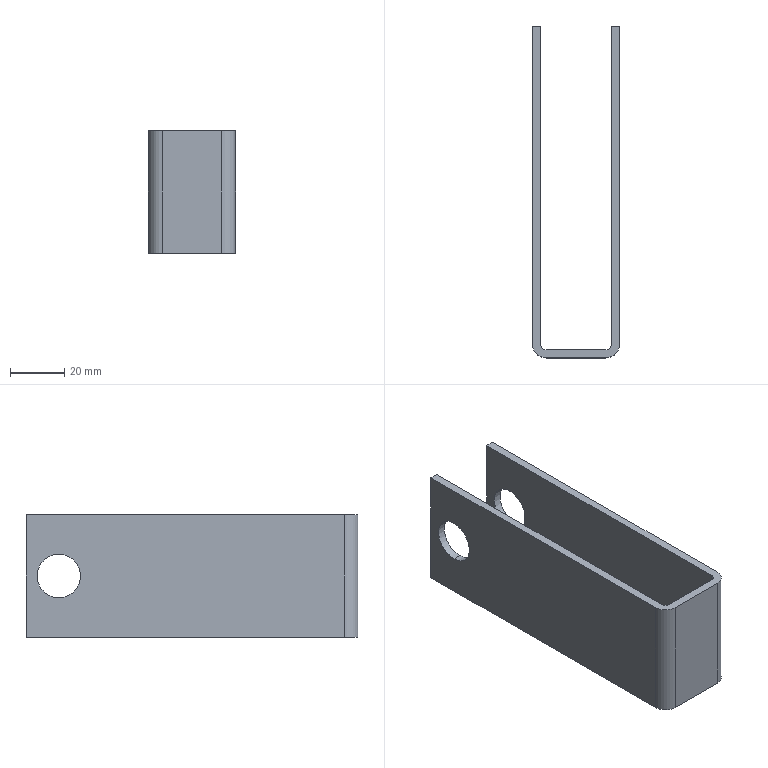Part | SolidWorks | features Extrusion 1, ICE 1 | 1 solid | 18 faces | box 32 x 122 x 45 mm | volume 34838 mm3 | plane 10 | cylinder 8 | commonest cylinder face diameters 16 x4 4 x2 10 x2
STEP:
#1=CARTESIAN_POINT('',(29.,-12.,30.5));
#2=VERTEX_POINT('',#1);
#3=CARTESIAN_POINT('',(29.,-12.,14.5));
#4=VERTEX_POINT('',#3);
#5=CARTESIAN_POINT('',(29.,-12.,22.5));
#6=DIRECTION('',(1.,0.,0.));
#7=DIRECTION('',(0.,1.,0.));
#8=AXIS2_PLACEMENT_3D('',#5,#6,#7);
#9=CIRCLE('',#8,8.);
#10=EDGE_CURVE('',#2,#4,#9,.T.);
#11=ORIENTED_EDGE('',*,*,#10,.F.);
#12=CARTESIAN_POINT('',(32.,-12.,30.5));
#13=VERTEX_POINT('',#12);
#14=CARTESIAN_POINT('',(0.,-12.,30.5));
#15=DIRECTION('',(1.,0.,0.));
#16=VECTOR('',#15,1000.);
#17=LINE('',#14,#16);
#18=EDGE_CURVE('',#2,#13,#17,.T.);
#19=ORIENTED_EDGE('',*,*,#18,.T.);
#20=CARTESIAN_POINT('',(32.,-12.,14.5));
#21=VERTEX_POINT('',#20);
#22=CARTESIAN_POINT('',(32.,-12.,22.5));
#23=DIRECTION('',(1.,0.,0.));
#24=DIRECTION('',(0.,0.,-1.));
#25=AXIS2_PLACEMENT_3D('',#22,#23,#24);
#26=CIRCLE('',#25,8.);
#27=EDGE_CURVE('',#13,#21,#26,.T.);
#28=ORIENTED_EDGE('',*,*,#27,.T.);
#29=CARTESIAN_POINT('',(0.,-12.,14.5));
#30=DIRECTION('',(1.,0.,0.));
#31=VECTOR('',#30,1000.);
#32=LINE('',#29,#31);
#33=EDGE_CURVE('',#4,#21,#32,.T.);
#34=ORIENTED_EDGE('',*,*,#33,.F.);
#35=EDGE_LOOP('',(#11,#19,#28,#34));
#36=FACE_OUTER_BOUND('',#35,.T.);
#37=CARTESIAN_POINT('',(0.,-12.,22.5));
#38=DIRECTION('',(1.,0.,0.));
#39=DIRECTION('',(0.,0.,-1.));
#40=AXIS2_PLACEMENT_3D('',#37,#38,#39);
#41=CYLINDRICAL_SURFACE('',#40,8.);
#42=ADVANCED_FACE('',(#36),#41,.F.);
#43=CARTESIAN_POINT('',(0.,-12.,30.5));
#44=VERTEX_POINT('',#43);
#45=CARTESIAN_POINT('',(0.,-12.,14.5));
#46=VERTEX_POINT('',#45);
#47=CARTESIAN_POINT('',(0.,-12.,22.5));
#48=DIRECTION('',(1.,0.,0.));
#49=DIRECTION('',(0.,0.,-1.));
#50=AXIS2_PLACEMENT_3D('',#47,#48,#49);
#51=CIRCLE('',#50,8.);
#52=EDGE_CURVE('',#44,#46,#51,.T.);
#53=ORIENTED_EDGE('',*,*,#52,.F.);
#54=CARTESIAN_POINT('',(3.,-12.,30.5));
#55=VERTEX_POINT('',#54);
#56=CARTESIAN_POINT('',(0.,-12.,30.5));
#57=DIRECTION('',(1.,0.,0.));
#58=VECTOR('',#57,1000.);
#59=LINE('',#56,#58);
#60=EDGE_CURVE('',#44,#55,#59,.T.);
#61=ORIENTED_EDGE('',*,*,#60,.T.);
#62=CARTESIAN_POINT('',(3.,-12.,14.5));
#63=VERTEX_POINT('',#62);
#64=CARTESIAN_POINT('',(3.,-12.,22.5));
#65=DIRECTION('',(-1.,0.,0.));
#66=DIRECTION('',(0.,-1.,0.));
#67=AXIS2_PLACEMENT_3D('',#64,#65,#66);
#68=CIRCLE('',#67,8.);
#69=EDGE_CURVE('',#63,#55,#68,.T.);
#70=ORIENTED_EDGE('',*,*,#69,.F.);
#71=CARTESIAN_POINT('',(0.,-12.,14.5));
#72=DIRECTION('',(1.,0.,0.));
#73=VECTOR('',#72,1000.);
#74=LINE('',#71,#73);
#75=EDGE_CURVE('',#46,#63,#74,.T.);
#76=ORIENTED_EDGE('',*,*,#75,.F.);
#77=EDGE_LOOP('',(#53,#61,#70,#76));
#78=FACE_OUTER_BOUND('',#77,.T.);
#79=CARTESIAN_POINT('',(0.,-12.,22.5));
#80=DIRECTION('',(1.,0.,0.));
#81=DIRECTION('',(0.,0.,-1.));
#82=AXIS2_PLACEMENT_3D('',#79,#80,#81);
#83=CYLINDRICAL_SURFACE('',#82,8.);
#84=ADVANCED_FACE('',(#78),#83,.F.);
#85=CARTESIAN_POINT('',(3.,0.,0.));
#86=VERTEX_POINT('',#85);
#87=CARTESIAN_POINT('',(0.,0.,0.));
#88=VERTEX_POINT('',#87);
#89=CARTESIAN_POINT('',(3.,0.,0.));
#90=DIRECTION('',(-1.,0.,0.));
#91=VECTOR('',#90,1000.);
#92=LINE('',#89,#91);
#93=EDGE_CURVE('',#86,#88,#92,.T.);
#94=ORIENTED_EDGE('',*,*,#93,.T.);
#95=CARTESIAN_POINT('',(0.,0.,45.));
#96=VERTEX_POINT('',#95);
#97=CARTESIAN_POINT('',(0.,0.,45.));
#98=DIRECTION('',(0.,0.,-1.));
#99=VECTOR('',#98,1000.);
#100=LINE('',#97,#99);
#101=EDGE_CURVE('',#96,#88,#100,.T.);
#102=ORIENTED_EDGE('',*,*,#101,.F.);
#103=CARTESIAN_POINT('',(3.,0.,45.));
#104=VERTEX_POINT('',#103);
#105=CARTESIAN_POINT('',(3.,0.,45.));
#106=DIRECTION('',(-1.,0.,0.));
#107=VECTOR('',#106,1000.);
#108=LINE('',#105,#107);
#109=EDGE_CURVE('',#104,#96,#108,.T.);
#110=ORIENTED_EDGE('',*,*,#109,.F.);
#111=CARTESIAN_POINT('',(3.,0.,45.));
#112=DIRECTION('',(0.,0.,-1.));
#113=VECTOR('',#112,1000.);
#114=LINE('',#111,#113);
#115=EDGE_CURVE('',#104,#86,#114,.T.);
#116=ORIENTED_EDGE('',*,*,#115,.T.);
#117=EDGE_LOOP('',(#94,#102,#110,#116));
#118=FACE_OUTER_BOUND('',#117,.T.);
#119=CARTESIAN_POINT('',(3.,0.,45.));
#120=DIRECTION('',(0.,-1.,0.));
#121=DIRECTION('',(0.,0.,-1.));
#122=AXIS2_PLACEMENT_3D('',#119,#120,#121);
#123=PLANE('',#122);
#124=ADVANCED_FACE('',(#118),#123,.F.);
#125=CARTESIAN_POINT('',(0.,-12.,22.5));
#126=DIRECTION('',(1.,0.,0.));
#127=DIRECTION('',(0.,0.,-1.));
#128=AXIS2_PLACEMENT_3D('',#125,#126,#127);
#129=CIRCLE('',#128,8.);
#130=EDGE_CURVE('',#46,#44,#129,.T.);
#131=ORIENTED_EDGE('',*,*,#130,.T.);
#132=ORIENTED_EDGE('',*,*,#52,.T.);
#133=EDGE_LOOP('',(#131,#132));
#134=FACE_BOUND('',#133,.T.);
#135=CARTESIAN_POINT('',(0.,-117.,0.));
#136=VERTEX_POINT('',#135);
#137=CARTESIAN_POINT('',(0.,0.,0.));
#138=DIRECTION('',(0.,-1.,0.));
#139=VECTOR('',#138,1000.);
#140=LINE('',#137,#139);
#141=EDGE_CURVE('',#88,#136,#140,.T.);
#142=ORIENTED_EDGE('',*,*,#141,.T.);
#143=CARTESIAN_POINT('',(0.,-117.,45.));
#144=VERTEX_POINT('',#143);
#145=CARTESIAN_POINT('',(0.,-117.,45.));
#146=DIRECTION('',(0.,0.,-1.));
#147=VECTOR('',#146,1000.);
#148=LINE('',#145,#147);
#149=EDGE_CURVE('',#144,#136,#148,.T.);
#150=ORIENTED_EDGE('',*,*,#149,.F.);
#151=CARTESIAN_POINT('',(0.,0.,45.));
#152=DIRECTION('',(0.,-1.,0.));
#153=VECTOR('',#152,1000.);
#154=LINE('',#151,#153);
#155=EDGE_CURVE('',#96,#144,#154,.T.);
#156=ORIENTED_EDGE('',*,*,#155,.F.);
#157=ORIENTED_EDGE('',*,*,#101,.T.);
#158=EDGE_LOOP('',(#142,#150,#156,#157));
#159=FACE_OUTER_BOUND('',#158,.T.);
#160=CARTESIAN_POINT('',(0.,0.,45.));
#161=DIRECTION('',(1.,0.,0.));
#162=DIRECTION('',(0.,1.,0.));
#163=AXIS2_PLACEMENT_3D('',#160,#161,#162);
#164=PLANE('',#163);
#165=ADVANCED_FACE('',(#134,#159),#164,.F.);
#166=CARTESIAN_POINT('',(5.,-122.,0.));
#167=VERTEX_POINT('',#166);
#168=CARTESIAN_POINT('',(5.,-117.,0.));
#169=DIRECTION('',(0.,0.,1.));
#170=DIRECTION('',(1.,0.,0.));
#171=AXIS2_PLACEMENT_3D('',#168,#169,#170);
#172=CIRCLE('',#171,5.);
#173=EDGE_CURVE('',#136,#167,#172,.T.);
#174=ORIENTED_EDGE('',*,*,#173,.T.);
#175=CARTESIAN_POINT('',(5.,-122.,45.));
#176=VERTEX_POINT('',#175);
#177=CARTESIAN_POINT('',(5.,-122.,45.));
#178=DIRECTION('',(0.,0.,-1.));
#179=VECTOR('',#178,1000.);
#180=LINE('',#177,#179);
#181=EDGE_CURVE('',#176,#167,#180,.T.);
#182=ORIENTED_EDGE('',*,*,#181,.F.);
#183=CARTESIAN_POINT('',(5.,-117.,45.));
#184=DIRECTION('',(0.,0.,1.));
#185=DIRECTION('',(1.,0.,0.));
#186=AXIS2_PLACEMENT_3D('',#183,#184,#185);
#187=CIRCLE('',#186,5.);
#188=EDGE_CURVE('',#144,#176,#187,.T.);
#189=ORIENTED_EDGE('',*,*,#188,.F.);
#190=ORIENTED_EDGE('',*,*,#149,.T.);
#191=EDGE_LOOP('',(#174,#182,#189,#190));
#192=FACE_OUTER_BOUND('',#191,.T.);
#193=CARTESIAN_POINT('',(5.,-117.,45.));
#194=DIRECTION('',(0.,0.,-1.));
#195=DIRECTION('',(-1.,0.,0.));
#196=AXIS2_PLACEMENT_3D('',#193,#194,#195);
#197=CYLINDRICAL_SURFACE('',#196,5.);
#198=ADVANCED_FACE('',(#192),#197,.T.);
#199=CARTESIAN_POINT('',(27.,-122.,0.));
#200=VERTEX_POINT('',#199);
#201=CARTESIAN_POINT('',(5.,-122.,0.));
#202=DIRECTION('',(1.,0.,0.));
#203=VECTOR('',#202,1000.);
#204=LINE('',#201,#203);
#205=EDGE_CURVE('',#167,#200,#204,.T.);
#206=ORIENTED_EDGE('',*,*,#205,.T.);
#207=CARTESIAN_POINT('',(27.,-122.,45.));
#208=VERTEX_POINT('',#207);
#209=CARTESIAN_POINT('',(27.,-122.,45.));
#210=DIRECTION('',(0.,0.,-1.));
#211=VECTOR('',#210,1000.);
#212=LINE('',#209,#211);
#213=EDGE_CURVE('',#208,#200,#212,.T.);
#214=ORIENTED_EDGE('',*,*,#213,.F.);
#215=CARTESIAN_POINT('',(5.,-122.,45.));
#216=DIRECTION('',(1.,0.,0.));
#217=VECTOR('',#216,1000.);
#218=LINE('',#215,#217);
#219=EDGE_CURVE('',#176,#208,#218,.T.);
#220=ORIENTED_EDGE('',*,*,#219,.F.);
#221=ORIENTED_EDGE('',*,*,#181,.T.);
#222=EDGE_LOOP('',(#206,#214,#220,#221));
#223=FACE_OUTER_BOUND('',#222,.T.);
#224=CARTESIAN_POINT('',(5.,-122.,45.));
#225=DIRECTION('',(0.,1.,0.));
#226=DIRECTION('',(0.,0.,1.));
#227=AXIS2_PLACEMENT_3D('',#224,#225,#226);
#228=PLANE('',#227);
#229=ADVANCED_FACE('',(#223),#228,.F.);
#230=CARTESIAN_POINT('',(32.,-117.,0.));
#231=VERTEX_POINT('',#230);
#232=CARTESIAN_POINT('',(27.,-117.,0.));
#233=DIRECTION('',(0.,0.,1.));
#234=DIRECTION('',(1.,0.,0.));
#235=AXIS2_PLACEMENT_3D('',#232,#233,#234);
#236=CIRCLE('',#235,5.);
#237=EDGE_CURVE('',#200,#231,#236,.T.);
#238=ORIENTED_EDGE('',*,*,#237,.T.);
#239=CARTESIAN_POINT('',(32.,-117.,45.));
#240=VERTEX_POINT('',#239);
#241=CARTESIAN_POINT('',(32.,-117.,45.));
#242=DIRECTION('',(0.,0.,-1.));
#243=VECTOR('',#242,1000.);
#244=LINE('',#241,#243);
#245=EDGE_CURVE('',#240,#231,#244,.T.);
#246=ORIENTED_EDGE('',*,*,#245,.F.);
#247=CARTESIAN_POINT('',(27.,-117.,45.));
#248=DIRECTION('',(0.,0.,1.));
#249=DIRECTION('',(1.,0.,0.));
#250=AXIS2_PLACEMENT_3D('',#247,#248,#249);
#251=CIRCLE('',#250,5.);
#252=EDGE_CURVE('',#208,#240,#251,.T.);
#253=ORIENTED_EDGE('',*,*,#252,.F.);
#254=ORIENTED_EDGE('',*,*,#213,.T.);
#255=EDGE_LOOP('',(#238,#246,#253,#254));
#256=FACE_OUTER_BOUND('',#255,.T.);
#257=CARTESIAN_POINT('',(27.,-117.,45.));
#258=DIRECTION('',(0.,0.,-1.));
#259=DIRECTION('',(-1.,0.,0.));
#260=AXIS2_PLACEMENT_3D('',#257,#258,#259);
#261=CYLINDRICAL_SURFACE('',#260,5.);
#262=ADVANCED_FACE('',(#256),#261,.T.);
#263=CARTESIAN_POINT('',(32.,-12.,22.5));
#264=DIRECTION('',(1.,0.,0.));
#265=DIRECTION('',(0.,0.,-1.));
#266=AXIS2_PLACEMENT_3D('',#263,#264,#265);
#267=CIRCLE('',#266,8.);
#268=EDGE_CURVE('',#21,#13,#267,.T.);
#269=ORIENTED_EDGE('',*,*,#268,.F.);
#270=ORIENTED_EDGE('',*,*,#27,.F.);
#271=EDGE_LOOP('',(#269,#270));
#272=FACE_BOUND('',#271,.T.);
#273=CARTESIAN_POINT('',(32.,0.,0.));
#274=VERTEX_POINT('',#273);
#275=CARTESIAN_POINT('',(32.,-117.,0.));
#276=DIRECTION('',(0.,1.,0.));
#277=VECTOR('',#276,1000.);
#278=LINE('',#275,#277);
#279=EDGE_CURVE('',#231,#274,#278,.T.);
#280=ORIENTED_EDGE('',*,*,#279,.T.);
#281=CARTESIAN_POINT('',(32.,0.,45.));
#282=VERTEX_POINT('',#281);
#283=CARTESIAN_POINT('',(32.,0.,45.));
#284=DIRECTION('',(0.,0.,-1.));
#285=VECTOR('',#284,1000.);
#286=LINE('',#283,#285);
#287=EDGE_CURVE('',#282,#274,#286,.T.);
#288=ORIENTED_EDGE('',*,*,#287,.F.);
#289=CARTESIAN_POINT('',(32.,-117.,45.));
#290=DIRECTION('',(0.,1.,0.));
#291=VECTOR('',#290,1000.);
#292=LINE('',#289,#291);
#293=EDGE_CURVE('',#240,#282,#292,.T.);
#294=ORIENTED_EDGE('',*,*,#293,.F.);
#295=ORIENTED_EDGE('',*,*,#245,.T.);
#296=EDGE_LOOP('',(#280,#288,#294,#295));
#297=FACE_OUTER_BOUND('',#296,.T.);
#298=CARTESIAN_POINT('',(32.,-117.,45.));
#299=DIRECTION('',(-1.,0.,0.));
#300=DIRECTION('',(0.,-1.,0.));
#301=AXIS2_PLACEMENT_3D('',#298,#299,#300);
#302=PLANE('',#301);
#303=ADVANCED_FACE('',(#272,#297),#302,.F.);
#304=CARTESIAN_POINT('',(29.,0.,0.));
#305=VERTEX_POINT('',#304);
#306=CARTESIAN_POINT('',(29.,0.,0.));
#307=DIRECTION('',(-1.,0.,0.));
#308=VECTOR('',#307,1000.);
#309=LINE('',#306,#308);
#310=EDGE_CURVE('',#274,#305,#309,.T.);
#311=ORIENTED_EDGE('',*,*,#310,.T.);
#312=CARTESIAN_POINT('',(29.,0.,45.));
#313=VERTEX_POINT('',#312);
#314=CARTESIAN_POINT('',(29.,0.,45.));
#315=DIRECTION('',(0.,0.,-1.));
#316=VECTOR('',#315,1000.);
#317=LINE('',#314,#316);
#318=EDGE_CURVE('',#313,#305,#317,.T.);
#319=ORIENTED_EDGE('',*,*,#318,.F.);
#320=CARTESIAN_POINT('',(29.,0.,45.));
#321=DIRECTION('',(-1.,0.,0.));
#322=VECTOR('',#321,1000.);
#323=LINE('',#320,#322);
#324=EDGE_CURVE('',#282,#313,#323,.T.);
#325=ORIENTED_EDGE('',*,*,#324,.F.);
#326=ORIENTED_EDGE('',*,*,#287,.T.);
#327=EDGE_LOOP('',(#311,#319,#325,#326));
#328=FACE_OUTER_BOUND('',#327,.T.);
#329=CARTESIAN_POINT('',(29.,0.,45.));
#330=DIRECTION('',(0.,-1.,0.));
#331=DIRECTION('',(1.,0.,0.));
#332=AXIS2_PLACEMENT_3D('',#329,#330,#331);
#333=PLANE('',#332);
#334=ADVANCED_FACE('',(#328),#333,.F.);
#335=CARTESIAN_POINT('',(29.,-12.,22.5));
#336=DIRECTION('',(1.,0.,0.));
#337=DIRECTION('',(0.,1.,0.));
#338=AXIS2_PLACEMENT_3D('',#335,#336,#337);
#339=CIRCLE('',#338,8.);
#340=EDGE_CURVE('',#4,#2,#339,.T.);
#341=ORIENTED_EDGE('',*,*,#340,.T.);
#342=ORIENTED_EDGE('',*,*,#10,.T.);
#343=EDGE_LOOP('',(#341,#342));
#344=FACE_BOUND('',#343,.T.);
#345=CARTESIAN_POINT('',(29.,-117.,0.));
#346=VERTEX_POINT('',#345);
#347=CARTESIAN_POINT('',(29.,-117.,0.));
#348=DIRECTION('',(0.,-1.,0.));
#349=VECTOR('',#348,1000.);
#350=LINE('',#347,#349);
#351=EDGE_CURVE('',#305,#346,#350,.T.);
#352=ORIENTED_EDGE('',*,*,#351,.T.);
#353=CARTESIAN_POINT('',(29.,-117.,45.));
#354=VERTEX_POINT('',#353);
#355=CARTESIAN_POINT('',(29.,-117.,45.));
#356=DIRECTION('',(0.,0.,-1.));
#357=VECTOR('',#356,1000.);
#358=LINE('',#355,#357);
#359=EDGE_CURVE('',#354,#346,#358,.T.);
#360=ORIENTED_EDGE('',*,*,#359,.F.);
#361=CARTESIAN_POINT('',(29.,-117.,45.));
#362=DIRECTION('',(0.,-1.,0.));
#363=VECTOR('',#362,1000.);
#364=LINE('',#361,#363);
#365=EDGE_CURVE('',#313,#354,#364,.T.);
#366=ORIENTED_EDGE('',*,*,#365,.F.);
#367=ORIENTED_EDGE('',*,*,#318,.T.);
#368=EDGE_LOOP('',(#352,#360,#366,#367));
#369=FACE_OUTER_BOUND('',#368,.T.);
#370=CARTESIAN_POINT('',(29.,-117.,45.));
#371=DIRECTION('',(1.,0.,0.));
#372=DIRECTION('',(0.,1.,0.));
#373=AXIS2_PLACEMENT_3D('',#370,#371,#372);
#374=PLANE('',#373);
#375=ADVANCED_FACE('',(#344,#369),#374,.F.);
#376=CARTESIAN_POINT('',(27.,-119.,0.));
#377=VERTEX_POINT('',#376);
#378=CARTESIAN_POINT('',(27.,-117.,0.));
#379=DIRECTION('',(0.,0.,-1.));
#380=DIRECTION('',(1.,0.,0.));
#381=AXIS2_PLACEMENT_3D('',#378,#379,#380);
#382=CIRCLE('',#381,2.);
#383=EDGE_CURVE('',#346,#377,#382,.T.);
#384=ORIENTED_EDGE('',*,*,#383,.T.);
#385=CARTESIAN_POINT('',(27.,-119.,45.));
#386=VERTEX_POINT('',#385);
#387=CARTESIAN_POINT('',(27.,-119.,45.));
#388=DIRECTION('',(0.,0.,-1.));
#389=VECTOR('',#388,1000.);
#390=LINE('',#387,#389);
#391=EDGE_CURVE('',#386,#377,#390,.T.);
#392=ORIENTED_EDGE('',*,*,#391,.F.);
#393=CARTESIAN_POINT('',(27.,-117.,45.));
#394=DIRECTION('',(0.,0.,-1.));
#395=DIRECTION('',(1.,0.,0.));
#396=AXIS2_PLACEMENT_3D('',#393,#394,#395);
#397=CIRCLE('',#396,2.);
#398=EDGE_CURVE('',#354,#386,#397,.T.);
#399=ORIENTED_EDGE('',*,*,#398,.F.);
#400=ORIENTED_EDGE('',*,*,#359,.T.);
#401=EDGE_LOOP('',(#384,#392,#399,#400));
#402=FACE_OUTER_BOUND('',#401,.T.);
#403=CARTESIAN_POINT('',(27.,-117.,45.));
#404=DIRECTION('',(0.,0.,-1.));
#405=DIRECTION('',(-1.,0.,0.));
#406=AXIS2_PLACEMENT_3D('',#403,#404,#405);
#407=CYLINDRICAL_SURFACE('',#406,2.);
#408=ADVANCED_FACE('',(#402),#407,.F.);
#409=CARTESIAN_POINT('',(5.,-119.,0.));
#410=VERTEX_POINT('',#409);
#411=CARTESIAN_POINT('',(5.,-119.,0.));
#412=DIRECTION('',(-1.,0.,0.));
#413=VECTOR('',#412,1000.);
#414=LINE('',#411,#413);
#415=EDGE_CURVE('',#377,#410,#414,.T.);
#416=ORIENTED_EDGE('',*,*,#415,.T.);
#417=CARTESIAN_POINT('',(5.,-119.,45.));
#418=VERTEX_POINT('',#417);
#419=CARTESIAN_POINT('',(5.,-119.,45.));
#420=DIRECTION('',(0.,0.,-1.));
#421=VECTOR('',#420,1000.);
#422=LINE('',#419,#421);
#423=EDGE_CURVE('',#418,#410,#422,.T.);
#424=ORIENTED_EDGE('',*,*,#423,.F.);
#425=CARTESIAN_POINT('',(5.,-119.,45.));
#426=DIRECTION('',(-1.,0.,0.));
#427=VECTOR('',#426,1000.);
#428=LINE('',#425,#427);
#429=EDGE_CURVE('',#386,#418,#428,.T.);
#430=ORIENTED_EDGE('',*,*,#429,.F.);
#431=ORIENTED_EDGE('',*,*,#391,.T.);
#432=EDGE_LOOP('',(#416,#424,#430,#431));
#433=FACE_OUTER_BOUND('',#432,.T.);
#434=CARTESIAN_POINT('',(5.,-119.,45.));
#435=DIRECTION('',(0.,-1.,0.));
#436=DIRECTION('',(0.,0.,-1.));
#437=AXIS2_PLACEMENT_3D('',#434,#435,#436);
#438=PLANE('',#437);
#439=ADVANCED_FACE('',(#433),#438,.F.);
#440=CARTESIAN_POINT('',(3.,-117.,0.));
#441=VERTEX_POINT('',#440);
#442=CARTESIAN_POINT('',(5.,-117.,0.));
#443=DIRECTION('',(0.,0.,-1.));
#444=DIRECTION('',(1.,0.,0.));
#445=AXIS2_PLACEMENT_3D('',#442,#443,#444);
#446=CIRCLE('',#445,2.);
#447=EDGE_CURVE('',#410,#441,#446,.T.);
#448=ORIENTED_EDGE('',*,*,#447,.T.);
#449=CARTESIAN_POINT('',(3.,-117.,45.));
#450=VERTEX_POINT('',#449);
#451=CARTESIAN_POINT('',(3.,-117.,45.));
#452=DIRECTION('',(0.,0.,-1.));
#453=VECTOR('',#452,1000.);
#454=LINE('',#451,#453);
#455=EDGE_CURVE('',#450,#441,#454,.T.);
#456=ORIENTED_EDGE('',*,*,#455,.F.);
#457=CARTESIAN_POINT('',(5.,-117.,45.));
#458=DIRECTION('',(0.,0.,-1.));
#459=DIRECTION('',(1.,0.,0.));
#460=AXIS2_PLACEMENT_3D('',#457,#458,#459);
#461=CIRCLE('',#460,2.);
#462=EDGE_CURVE('',#418,#450,#461,.T.);
#463=ORIENTED_EDGE('',*,*,#462,.F.);
#464=ORIENTED_EDGE('',*,*,#423,.T.);
#465=EDGE_LOOP('',(#448,#456,#463,#464));
#466=FACE_OUTER_BOUND('',#465,.T.);
#467=CARTESIAN_POINT('',(5.,-117.,45.));
#468=DIRECTION('',(0.,0.,-1.));
#469=DIRECTION('',(-1.,0.,0.));
#470=AXIS2_PLACEMENT_3D('',#467,#468,#469);
#471=CYLINDRICAL_SURFACE('',#470,2.);
#472=ADVANCED_FACE('',(#466),#471,.F.);
#473=ORIENTED_EDGE('',*,*,#69,.T.);
#474=CARTESIAN_POINT('',(3.,-12.,22.5));
#475=DIRECTION('',(-1.,0.,0.));
#476=DIRECTION('',(0.,-1.,0.));
#477=AXIS2_PLACEMENT_3D('',#474,#475,#476);
#478=CIRCLE('',#477,8.);
#479=EDGE_CURVE('',#55,#63,#478,.T.);
#480=ORIENTED_EDGE('',*,*,#479,.T.);
#481=EDGE_LOOP('',(#473,#480));
#482=FACE_BOUND('',#481,.T.);
#483=CARTESIAN_POINT('',(3.,0.,0.));
#484=DIRECTION('',(0.,1.,0.));
#485=VECTOR('',#484,1000.);
#486=LINE('',#483,#485);
#487=EDGE_CURVE('',#441,#86,#486,.T.);
#488=ORIENTED_EDGE('',*,*,#487,.T.);
#489=ORIENTED_EDGE('',*,*,#115,.F.);
#490=CARTESIAN_POINT('',(3.,0.,45.));
#491=DIRECTION('',(0.,1.,0.));
#492=VECTOR('',#491,1000.);
#493=LINE('',#490,#492);
#494=EDGE_CURVE('',#450,#104,#493,.T.);
#495=ORIENTED_EDGE('',*,*,#494,.F.);
#496=ORIENTED_EDGE('',*,*,#455,.T.);
#497=EDGE_LOOP('',(#488,#489,#495,#496));
#498=FACE_OUTER_BOUND('',#497,.T.);
#499=CARTESIAN_POINT('',(3.,0.,45.));
#500=DIRECTION('',(-1.,0.,0.));
#501=DIRECTION('',(0.,-1.,0.));
#502=AXIS2_PLACEMENT_3D('',#499,#500,#501);
#503=PLANE('',#502);
#504=ADVANCED_FACE('',(#482,#498),#503,.F.);
#505=ORIENTED_EDGE('',*,*,#109,.T.);
#506=ORIENTED_EDGE('',*,*,#155,.T.);
#507=ORIENTED_EDGE('',*,*,#188,.T.);
#508=ORIENTED_EDGE('',*,*,#219,.T.);
#509=ORIENTED_EDGE('',*,*,#252,.T.);
#510=ORIENTED_EDGE('',*,*,#293,.T.);
#511=ORIENTED_EDGE('',*,*,#324,.T.);
#512=ORIENTED_EDGE('',*,*,#365,.T.);
#513=ORIENTED_EDGE('',*,*,#398,.T.);
#514=ORIENTED_EDGE('',*,*,#429,.T.);
#515=ORIENTED_EDGE('',*,*,#462,.T.);
#516=ORIENTED_EDGE('',*,*,#494,.T.);
#517=EDGE_LOOP('',(#505,#506,#507,#508,#509,#510,#511,#512,#513,#514,#515,#516));
#518=FACE_OUTER_BOUND('',#517,.T.);
#519=CARTESIAN_POINT('',(5.,-117.,45.));
#520=DIRECTION('',(0.,0.,1.));
#521=DIRECTION('',(1.,0.,0.));
#522=AXIS2_PLACEMENT_3D('',#519,#520,#521);
#523=PLANE('',#522);
#524=ADVANCED_FACE('',(#518),#523,.T.);
#525=ORIENTED_EDGE('',*,*,#93,.F.);
#526=ORIENTED_EDGE('',*,*,#487,.F.);
#527=ORIENTED_EDGE('',*,*,#447,.F.);
#528=ORIENTED_EDGE('',*,*,#415,.F.);
#529=ORIENTED_EDGE('',*,*,#383,.F.);
#530=ORIENTED_EDGE('',*,*,#351,.F.);
#531=ORIENTED_EDGE('',*,*,#310,.F.);
#532=ORIENTED_EDGE('',*,*,#279,.F.);
#533=ORIENTED_EDGE('',*,*,#237,.F.);
#534=ORIENTED_EDGE('',*,*,#205,.F.);
#535=ORIENTED_EDGE('',*,*,#173,.F.);
#536=ORIENTED_EDGE('',*,*,#141,.F.);
#537=EDGE_LOOP('',(#525,#526,#527,#528,#529,#530,#531,#532,#533,#534,#535,#536));
#538=FACE_OUTER_BOUND('',#537,.T.);
#539=CARTESIAN_POINT('',(5.,-117.,0.));
#540=DIRECTION('',(0.,0.,1.));
#541=DIRECTION('',(1.,0.,0.));
#542=AXIS2_PLACEMENT_3D('',#539,#540,#541);
#543=PLANE('',#542);
#544=ADVANCED_FACE('',(#538),#543,.F.);
#545=ORIENTED_EDGE('',*,*,#60,.F.);
#546=ORIENTED_EDGE('',*,*,#130,.F.);
#547=ORIENTED_EDGE('',*,*,#75,.T.);
#548=ORIENTED_EDGE('',*,*,#479,.F.);
#549=EDGE_LOOP('',(#545,#546,#547,#548));
#550=FACE_OUTER_BOUND('',#549,.T.);
#551=CARTESIAN_POINT('',(0.,-12.,22.5));
#552=DIRECTION('',(1.,0.,0.));
#553=DIRECTION('',(0.,0.,-1.));
#554=AXIS2_PLACEMENT_3D('',#551,#552,#553);
#555=CYLINDRICAL_SURFACE('',#554,8.);
#556=ADVANCED_FACE('',(#550),#555,.F.);
#557=ORIENTED_EDGE('',*,*,#18,.F.);
#558=ORIENTED_EDGE('',*,*,#340,.F.);
#559=ORIENTED_EDGE('',*,*,#33,.T.);
#560=ORIENTED_EDGE('',*,*,#268,.T.);
#561=EDGE_LOOP('',(#557,#558,#559,#560));
#562=FACE_OUTER_BOUND('',#561,.T.);
#563=CARTESIAN_POINT('',(0.,-12.,22.5));
#564=DIRECTION('',(1.,0.,0.));
#565=DIRECTION('',(0.,0.,-1.));
#566=AXIS2_PLACEMENT_3D('',#563,#564,#565);
#567=CYLINDRICAL_SURFACE('',#566,8.);
#568=ADVANCED_FACE('',(#562),#567,.F.);
#569=CLOSED_SHELL('',(#42,#84,#124,#165,#198,#229,#262,#303,#334,#375,#408,#439,#472,#504,#524,#544,#556,#568));
#570=MANIFOLD_SOLID_BREP('',#569);
#571=CARTESIAN_POINT('',(0.,0.,0.));
#572=DIRECTION('',(0.,0.,1.));
#573=DIRECTION('',(1.,0.,0.));
#574=AXIS2_PLACEMENT_3D('',#571,#572,#573);
#575=(LENGTH_UNIT()NAMED_UNIT(*)SI_UNIT(.MILLI.,.METRE.));
#576=UNCERTAINTY_MEASURE_WITH_UNIT(LENGTH_MEASURE(0.00001),#575,'','');
#577=(NAMED_UNIT(*)PLANE_ANGLE_UNIT()SI_UNIT($,.RADIAN.));
#578=(NAMED_UNIT(*)SI_UNIT($,.STERADIAN.)SOLID_ANGLE_UNIT());
#579=(GEOMETRIC_REPRESENTATION_CONTEXT(3)GLOBAL_UNCERTAINTY_ASSIGNED_CONTEXT((#576))GLOBAL_UNIT_ASSIGNED_CONTEXT((#575,#577,#578))REPRESENTATION_CONTEXT('',''));
#580=ADVANCED_BREP_SHAPE_REPRESENTATION('',(#570,#574),#579);